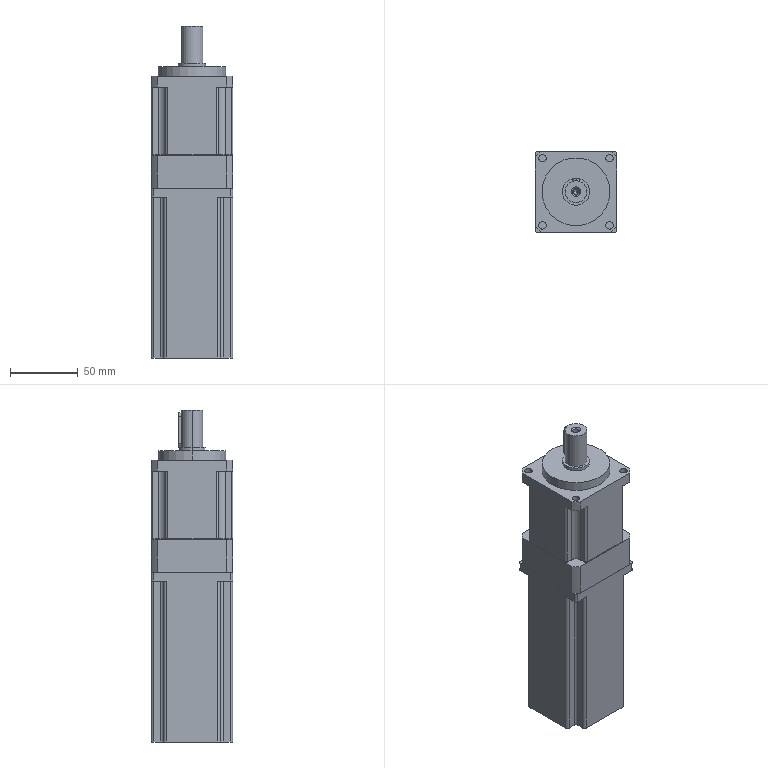Part | SolidWorks | 2 solids | 190 faces | box 60 x 60 x 244.5 mm | volume 699844 mm3 | cylinder 105 | plane 59 | cone 14 | torus 12 | commonest cylinder face diameters 4 x26 5.5 x16 5 x13 1 x12 70 x8 79 x8